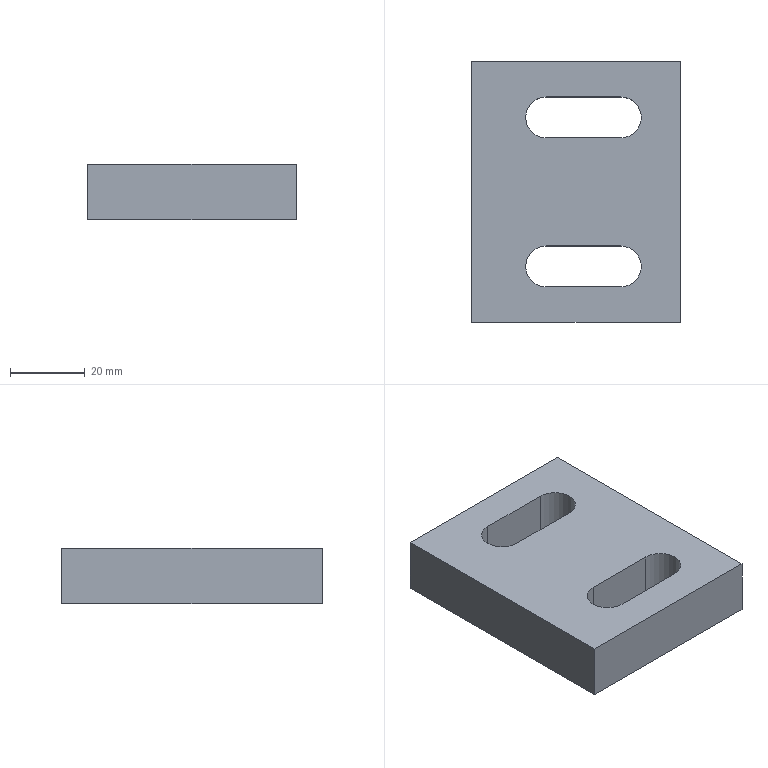Part | 1 solid | 16 faces | box 56 x 70 x 15 mm | volume 49349 mm3 | plane 10 | cylinder 6 | commonest cylinder face diameters 11 x6
STEP:
#1=CARTESIAN_POINT('',(-13.5,20.,15.));
#2=VERTEX_POINT('',#1);
#3=CARTESIAN_POINT('',(-8.,25.5,15.));
#4=VERTEX_POINT('',#3);
#5=CARTESIAN_POINT('',(-8.,20.,15.));
#6=DIRECTION('',(0.,0.,-1.));
#7=DIRECTION('',(-1.,0.,0.));
#8=AXIS2_PLACEMENT_3D('',#5,#6,#7);
#9=CIRCLE('',#8,5.5);
#10=EDGE_CURVE('',#2,#4,#9,.T.);
#11=ORIENTED_EDGE('',*,*,#10,.F.);
#12=CARTESIAN_POINT('',(-13.5,20.,0.));
#13=VERTEX_POINT('',#12);
#14=CARTESIAN_POINT('',(-13.5,20.,15.));
#15=DIRECTION('',(0.,0.,-1.));
#16=VECTOR('',#15,1000.);
#17=LINE('',#14,#16);
#18=EDGE_CURVE('',#2,#13,#17,.T.);
#19=ORIENTED_EDGE('',*,*,#18,.T.);
#20=CARTESIAN_POINT('',(-8.,25.5,0.));
#21=VERTEX_POINT('',#20);
#22=CARTESIAN_POINT('',(-8.,20.,0.));
#23=DIRECTION('',(0.,0.,1.));
#24=DIRECTION('',(-1.,0.,0.));
#25=AXIS2_PLACEMENT_3D('',#22,#23,#24);
#26=CIRCLE('',#25,5.5);
#27=EDGE_CURVE('',#21,#13,#26,.T.);
#28=ORIENTED_EDGE('',*,*,#27,.F.);
#29=CARTESIAN_POINT('',(-8.,25.5,15.));
#30=DIRECTION('',(0.,0.,-1.));
#31=VECTOR('',#30,1000.);
#32=LINE('',#29,#31);
#33=EDGE_CURVE('',#4,#21,#32,.T.);
#34=ORIENTED_EDGE('',*,*,#33,.F.);
#35=EDGE_LOOP('',(#11,#19,#28,#34));
#36=FACE_OUTER_BOUND('',#35,.T.);
#37=CARTESIAN_POINT('',(-8.,20.,15.));
#38=DIRECTION('',(0.,0.,-1.));
#39=DIRECTION('',(-1.,0.,0.));
#40=AXIS2_PLACEMENT_3D('',#37,#38,#39);
#41=CYLINDRICAL_SURFACE('',#40,5.5);
#42=ADVANCED_FACE('',(#36),#41,.F.);
#43=CARTESIAN_POINT('',(-13.5,-20.,15.));
#44=VERTEX_POINT('',#43);
#45=CARTESIAN_POINT('',(-8.,-14.5,15.));
#46=VERTEX_POINT('',#45);
#47=CARTESIAN_POINT('',(-8.,-20.,15.));
#48=DIRECTION('',(0.,0.,-1.));
#49=DIRECTION('',(1.,0.,0.));
#50=AXIS2_PLACEMENT_3D('',#47,#48,#49);
#51=CIRCLE('',#50,5.5);
#52=EDGE_CURVE('',#44,#46,#51,.T.);
#53=ORIENTED_EDGE('',*,*,#52,.F.);
#54=CARTESIAN_POINT('',(-13.5,-20.,0.));
#55=VERTEX_POINT('',#54);
#56=CARTESIAN_POINT('',(-13.5,-20.,15.));
#57=DIRECTION('',(0.,0.,-1.));
#58=VECTOR('',#57,1000.);
#59=LINE('',#56,#58);
#60=EDGE_CURVE('',#44,#55,#59,.T.);
#61=ORIENTED_EDGE('',*,*,#60,.T.);
#62=CARTESIAN_POINT('',(-8.,-14.5,0.));
#63=VERTEX_POINT('',#62);
#64=CARTESIAN_POINT('',(-8.,-20.,0.));
#65=DIRECTION('',(0.,0.,1.));
#66=DIRECTION('',(-1.,0.,0.));
#67=AXIS2_PLACEMENT_3D('',#64,#65,#66);
#68=CIRCLE('',#67,5.5);
#69=EDGE_CURVE('',#63,#55,#68,.T.);
#70=ORIENTED_EDGE('',*,*,#69,.F.);
#71=CARTESIAN_POINT('',(-8.,-14.5,15.));
#72=DIRECTION('',(0.,0.,-1.));
#73=VECTOR('',#72,1000.);
#74=LINE('',#71,#73);
#75=EDGE_CURVE('',#46,#63,#74,.T.);
#76=ORIENTED_EDGE('',*,*,#75,.F.);
#77=EDGE_LOOP('',(#53,#61,#70,#76));
#78=FACE_OUTER_BOUND('',#77,.T.);
#79=CARTESIAN_POINT('',(-8.,-20.,15.));
#80=DIRECTION('',(0.,0.,-1.));
#81=DIRECTION('',(-1.,0.,0.));
#82=AXIS2_PLACEMENT_3D('',#79,#80,#81);
#83=CYLINDRICAL_SURFACE('',#82,5.5);
#84=ADVANCED_FACE('',(#78),#83,.F.);
#85=CARTESIAN_POINT('',(28.,-35.,0.));
#86=VERTEX_POINT('',#85);
#87=CARTESIAN_POINT('',(28.,35.,0.));
#88=VERTEX_POINT('',#87);
#89=CARTESIAN_POINT('',(28.,35.,0.));
#90=DIRECTION('',(0.,1.,0.));
#91=VECTOR('',#90,1000.);
#92=LINE('',#89,#91);
#93=EDGE_CURVE('',#86,#88,#92,.T.);
#94=ORIENTED_EDGE('',*,*,#93,.T.);
#95=CARTESIAN_POINT('',(28.,35.,15.));
#96=VERTEX_POINT('',#95);
#97=CARTESIAN_POINT('',(28.,35.,15.));
#98=DIRECTION('',(0.,0.,-1.));
#99=VECTOR('',#98,1000.);
#100=LINE('',#97,#99);
#101=EDGE_CURVE('',#96,#88,#100,.T.);
#102=ORIENTED_EDGE('',*,*,#101,.F.);
#103=CARTESIAN_POINT('',(28.,-35.,15.));
#104=VERTEX_POINT('',#103);
#105=CARTESIAN_POINT('',(28.,35.,15.));
#106=DIRECTION('',(0.,1.,0.));
#107=VECTOR('',#106,1000.);
#108=LINE('',#105,#107);
#109=EDGE_CURVE('',#104,#96,#108,.T.);
#110=ORIENTED_EDGE('',*,*,#109,.F.);
#111=CARTESIAN_POINT('',(28.,-35.,15.));
#112=DIRECTION('',(0.,0.,-1.));
#113=VECTOR('',#112,1000.);
#114=LINE('',#111,#113);
#115=EDGE_CURVE('',#104,#86,#114,.T.);
#116=ORIENTED_EDGE('',*,*,#115,.T.);
#117=EDGE_LOOP('',(#94,#102,#110,#116));
#118=FACE_OUTER_BOUND('',#117,.T.);
#119=CARTESIAN_POINT('',(28.,35.,15.));
#120=DIRECTION('',(-1.,0.,0.));
#121=DIRECTION('',(0.,-1.,0.));
#122=AXIS2_PLACEMENT_3D('',#119,#120,#121);
#123=PLANE('',#122);
#124=ADVANCED_FACE('',(#118),#123,.F.);
#125=CARTESIAN_POINT('',(-28.,35.,0.));
#126=VERTEX_POINT('',#125);
#127=CARTESIAN_POINT('',(-28.,35.,0.));
#128=DIRECTION('',(-1.,0.,0.));
#129=VECTOR('',#128,1000.);
#130=LINE('',#127,#129);
#131=EDGE_CURVE('',#88,#126,#130,.T.);
#132=ORIENTED_EDGE('',*,*,#131,.T.);
#133=CARTESIAN_POINT('',(-28.,35.,15.));
#134=VERTEX_POINT('',#133);
#135=CARTESIAN_POINT('',(-28.,35.,15.));
#136=DIRECTION('',(0.,0.,-1.));
#137=VECTOR('',#136,1000.);
#138=LINE('',#135,#137);
#139=EDGE_CURVE('',#134,#126,#138,.T.);
#140=ORIENTED_EDGE('',*,*,#139,.F.);
#141=CARTESIAN_POINT('',(-28.,35.,15.));
#142=DIRECTION('',(-1.,0.,0.));
#143=VECTOR('',#142,1000.);
#144=LINE('',#141,#143);
#145=EDGE_CURVE('',#96,#134,#144,.T.);
#146=ORIENTED_EDGE('',*,*,#145,.F.);
#147=ORIENTED_EDGE('',*,*,#101,.T.);
#148=EDGE_LOOP('',(#132,#140,#146,#147));
#149=FACE_OUTER_BOUND('',#148,.T.);
#150=CARTESIAN_POINT('',(-28.,35.,15.));
#151=DIRECTION('',(0.,-1.,0.));
#152=DIRECTION('',(0.,0.,-1.));
#153=AXIS2_PLACEMENT_3D('',#150,#151,#152);
#154=PLANE('',#153);
#155=ADVANCED_FACE('',(#149),#154,.F.);
#156=CARTESIAN_POINT('',(-28.,-35.,0.));
#157=VERTEX_POINT('',#156);
#158=CARTESIAN_POINT('',(-28.,35.,0.));
#159=DIRECTION('',(0.,-1.,0.));
#160=VECTOR('',#159,1000.);
#161=LINE('',#158,#160);
#162=EDGE_CURVE('',#126,#157,#161,.T.);
#163=ORIENTED_EDGE('',*,*,#162,.T.);
#164=CARTESIAN_POINT('',(-28.,-35.,15.));
#165=VERTEX_POINT('',#164);
#166=CARTESIAN_POINT('',(-28.,-35.,15.));
#167=DIRECTION('',(0.,0.,-1.));
#168=VECTOR('',#167,1000.);
#169=LINE('',#166,#168);
#170=EDGE_CURVE('',#165,#157,#169,.T.);
#171=ORIENTED_EDGE('',*,*,#170,.F.);
#172=CARTESIAN_POINT('',(-28.,35.,15.));
#173=DIRECTION('',(0.,-1.,0.));
#174=VECTOR('',#173,1000.);
#175=LINE('',#172,#174);
#176=EDGE_CURVE('',#134,#165,#175,.T.);
#177=ORIENTED_EDGE('',*,*,#176,.F.);
#178=ORIENTED_EDGE('',*,*,#139,.T.);
#179=EDGE_LOOP('',(#163,#171,#177,#178));
#180=FACE_OUTER_BOUND('',#179,.T.);
#181=CARTESIAN_POINT('',(-28.,35.,15.));
#182=DIRECTION('',(1.,0.,0.));
#183=DIRECTION('',(0.,1.,0.));
#184=AXIS2_PLACEMENT_3D('',#181,#182,#183);
#185=PLANE('',#184);
#186=ADVANCED_FACE('',(#180),#185,.F.);
#187=CARTESIAN_POINT('',(-28.,-35.,0.));
#188=DIRECTION('',(1.,0.,0.));
#189=VECTOR('',#188,1000.);
#190=LINE('',#187,#189);
#191=EDGE_CURVE('',#157,#86,#190,.T.);
#192=ORIENTED_EDGE('',*,*,#191,.T.);
#193=ORIENTED_EDGE('',*,*,#115,.F.);
#194=CARTESIAN_POINT('',(-28.,-35.,15.));
#195=DIRECTION('',(1.,0.,0.));
#196=VECTOR('',#195,1000.);
#197=LINE('',#194,#196);
#198=EDGE_CURVE('',#165,#104,#197,.T.);
#199=ORIENTED_EDGE('',*,*,#198,.F.);
#200=ORIENTED_EDGE('',*,*,#170,.T.);
#201=EDGE_LOOP('',(#192,#193,#199,#200));
#202=FACE_OUTER_BOUND('',#201,.T.);
#203=CARTESIAN_POINT('',(-28.,-35.,15.));
#204=DIRECTION('',(0.,1.,0.));
#205=DIRECTION('',(0.,0.,1.));
#206=AXIS2_PLACEMENT_3D('',#203,#204,#205);
#207=PLANE('',#206);
#208=ADVANCED_FACE('',(#202),#207,.F.);
#209=CARTESIAN_POINT('',(12.,25.5,15.));
#210=VERTEX_POINT('',#209);
#211=CARTESIAN_POINT('',(12.,14.5,15.));
#212=VERTEX_POINT('',#211);
#213=CARTESIAN_POINT('',(12.,20.,15.));
#214=DIRECTION('',(0.,0.,-1.));
#215=DIRECTION('',(-1.,0.,0.));
#216=AXIS2_PLACEMENT_3D('',#213,#214,#215);
#217=CIRCLE('',#216,5.5);
#218=EDGE_CURVE('',#210,#212,#217,.T.);
#219=ORIENTED_EDGE('',*,*,#218,.T.);
#220=CARTESIAN_POINT('',(-8.,14.5,15.));
#221=VERTEX_POINT('',#220);
#222=CARTESIAN_POINT('',(12.,14.5,15.));
#223=DIRECTION('',(-1.,0.,0.));
#224=VECTOR('',#223,1000.);
#225=LINE('',#222,#224);
#226=EDGE_CURVE('',#212,#221,#225,.T.);
#227=ORIENTED_EDGE('',*,*,#226,.T.);
#228=CARTESIAN_POINT('',(-8.,20.,15.));
#229=DIRECTION('',(0.,0.,-1.));
#230=DIRECTION('',(-1.,0.,0.));
#231=AXIS2_PLACEMENT_3D('',#228,#229,#230);
#232=CIRCLE('',#231,5.5);
#233=EDGE_CURVE('',#221,#2,#232,.T.);
#234=ORIENTED_EDGE('',*,*,#233,.T.);
#235=ORIENTED_EDGE('',*,*,#10,.T.);
#236=CARTESIAN_POINT('',(12.,25.5,15.));
#237=DIRECTION('',(1.,0.,0.));
#238=VECTOR('',#237,1000.);
#239=LINE('',#236,#238);
#240=EDGE_CURVE('',#4,#210,#239,.T.);
#241=ORIENTED_EDGE('',*,*,#240,.T.);
#242=EDGE_LOOP('',(#219,#227,#234,#235,#241));
#243=FACE_BOUND('',#242,.T.);
#244=CARTESIAN_POINT('',(12.,-14.5,15.));
#245=VERTEX_POINT('',#244);
#246=CARTESIAN_POINT('',(12.,-25.5,15.));
#247=VERTEX_POINT('',#246);
#248=CARTESIAN_POINT('',(12.,-20.,15.));
#249=DIRECTION('',(0.,0.,-1.));
#250=DIRECTION('',(1.,0.,0.));
#251=AXIS2_PLACEMENT_3D('',#248,#249,#250);
#252=CIRCLE('',#251,5.5);
#253=EDGE_CURVE('',#245,#247,#252,.T.);
#254=ORIENTED_EDGE('',*,*,#253,.T.);
#255=CARTESIAN_POINT('',(-8.,-25.5,15.));
#256=VERTEX_POINT('',#255);
#257=CARTESIAN_POINT('',(12.,-25.5,15.));
#258=DIRECTION('',(-1.,0.,0.));
#259=VECTOR('',#258,1000.);
#260=LINE('',#257,#259);
#261=EDGE_CURVE('',#247,#256,#260,.T.);
#262=ORIENTED_EDGE('',*,*,#261,.T.);
#263=CARTESIAN_POINT('',(-8.,-20.,15.));
#264=DIRECTION('',(0.,0.,-1.));
#265=DIRECTION('',(1.,0.,0.));
#266=AXIS2_PLACEMENT_3D('',#263,#264,#265);
#267=CIRCLE('',#266,5.5);
#268=EDGE_CURVE('',#256,#44,#267,.T.);
#269=ORIENTED_EDGE('',*,*,#268,.T.);
#270=ORIENTED_EDGE('',*,*,#52,.T.);
#271=CARTESIAN_POINT('',(12.,-14.5,15.));
#272=DIRECTION('',(1.,0.,0.));
#273=VECTOR('',#272,1000.);
#274=LINE('',#271,#273);
#275=EDGE_CURVE('',#46,#245,#274,.T.);
#276=ORIENTED_EDGE('',*,*,#275,.T.);
#277=EDGE_LOOP('',(#254,#262,#269,#270,#276));
#278=FACE_BOUND('',#277,.T.);
#279=ORIENTED_EDGE('',*,*,#109,.T.);
#280=ORIENTED_EDGE('',*,*,#145,.T.);
#281=ORIENTED_EDGE('',*,*,#176,.T.);
#282=ORIENTED_EDGE('',*,*,#198,.T.);
#283=EDGE_LOOP('',(#279,#280,#281,#282));
#284=FACE_OUTER_BOUND('',#283,.T.);
#285=CARTESIAN_POINT('',(0.,0.,15.));
#286=DIRECTION('',(0.,0.,1.));
#287=DIRECTION('',(1.,0.,0.));
#288=AXIS2_PLACEMENT_3D('',#285,#286,#287);
#289=PLANE('',#288);
#290=ADVANCED_FACE('',(#243,#278,#284),#289,.T.);
#291=CARTESIAN_POINT('',(-8.,14.5,0.));
#292=VERTEX_POINT('',#291);
#293=CARTESIAN_POINT('',(12.,14.5,0.));
#294=VERTEX_POINT('',#293);
#295=CARTESIAN_POINT('',(0.,14.5,0.));
#296=DIRECTION('',(1.,0.,0.));
#297=VECTOR('',#296,1000.);
#298=LINE('',#295,#297);
#299=EDGE_CURVE('',#292,#294,#298,.T.);
#300=ORIENTED_EDGE('',*,*,#299,.T.);
#301=CARTESIAN_POINT('',(12.,25.5,0.));
#302=VERTEX_POINT('',#301);
#303=CARTESIAN_POINT('',(12.,20.,0.));
#304=DIRECTION('',(0.,0.,1.));
#305=DIRECTION('',(-1.,0.,0.));
#306=AXIS2_PLACEMENT_3D('',#303,#304,#305);
#307=CIRCLE('',#306,5.5);
#308=EDGE_CURVE('',#294,#302,#307,.T.);
#309=ORIENTED_EDGE('',*,*,#308,.T.);
#310=CARTESIAN_POINT('',(0.,25.5,0.));
#311=DIRECTION('',(-1.,0.,0.));
#312=VECTOR('',#311,1000.);
#313=LINE('',#310,#312);
#314=EDGE_CURVE('',#302,#21,#313,.T.);
#315=ORIENTED_EDGE('',*,*,#314,.T.);
#316=ORIENTED_EDGE('',*,*,#27,.T.);
#317=CARTESIAN_POINT('',(-8.,20.,0.));
#318=DIRECTION('',(0.,0.,1.));
#319=DIRECTION('',(-1.,0.,0.));
#320=AXIS2_PLACEMENT_3D('',#317,#318,#319);
#321=CIRCLE('',#320,5.5);
#322=EDGE_CURVE('',#13,#292,#321,.T.);
#323=ORIENTED_EDGE('',*,*,#322,.T.);
#324=EDGE_LOOP('',(#300,#309,#315,#316,#323));
#325=FACE_BOUND('',#324,.T.);
#326=CARTESIAN_POINT('',(-8.,-25.5,0.));
#327=VERTEX_POINT('',#326);
#328=CARTESIAN_POINT('',(12.,-25.5,0.));
#329=VERTEX_POINT('',#328);
#330=CARTESIAN_POINT('',(0.,-25.5,0.));
#331=DIRECTION('',(1.,0.,0.));
#332=VECTOR('',#331,1000.);
#333=LINE('',#330,#332);
#334=EDGE_CURVE('',#327,#329,#333,.T.);
#335=ORIENTED_EDGE('',*,*,#334,.T.);
#336=CARTESIAN_POINT('',(12.,-14.5,0.));
#337=VERTEX_POINT('',#336);
#338=CARTESIAN_POINT('',(12.,-20.,0.));
#339=DIRECTION('',(0.,0.,1.));
#340=DIRECTION('',(-1.,0.,0.));
#341=AXIS2_PLACEMENT_3D('',#338,#339,#340);
#342=CIRCLE('',#341,5.5);
#343=EDGE_CURVE('',#329,#337,#342,.T.);
#344=ORIENTED_EDGE('',*,*,#343,.T.);
#345=CARTESIAN_POINT('',(0.,-14.5,0.));
#346=DIRECTION('',(-1.,0.,0.));
#347=VECTOR('',#346,1000.);
#348=LINE('',#345,#347);
#349=EDGE_CURVE('',#337,#63,#348,.T.);
#350=ORIENTED_EDGE('',*,*,#349,.T.);
#351=ORIENTED_EDGE('',*,*,#69,.T.);
#352=CARTESIAN_POINT('',(-8.,-20.,0.));
#353=DIRECTION('',(0.,0.,1.));
#354=DIRECTION('',(-1.,0.,0.));
#355=AXIS2_PLACEMENT_3D('',#352,#353,#354);
#356=CIRCLE('',#355,5.5);
#357=EDGE_CURVE('',#55,#327,#356,.T.);
#358=ORIENTED_EDGE('',*,*,#357,.T.);
#359=EDGE_LOOP('',(#335,#344,#350,#351,#358));
#360=FACE_BOUND('',#359,.T.);
#361=ORIENTED_EDGE('',*,*,#93,.F.);
#362=ORIENTED_EDGE('',*,*,#191,.F.);
#363=ORIENTED_EDGE('',*,*,#162,.F.);
#364=ORIENTED_EDGE('',*,*,#131,.F.);
#365=EDGE_LOOP('',(#361,#362,#363,#364));
#366=FACE_OUTER_BOUND('',#365,.T.);
#367=CARTESIAN_POINT('',(0.,0.,0.));
#368=DIRECTION('',(0.,0.,1.));
#369=DIRECTION('',(1.,0.,0.));
#370=AXIS2_PLACEMENT_3D('',#367,#368,#369);
#371=PLANE('',#370);
#372=ADVANCED_FACE('',(#325,#360,#366),#371,.F.);
#373=CARTESIAN_POINT('',(12.,-25.5,15.));
#374=DIRECTION('',(0.,0.,-1.));
#375=VECTOR('',#374,1000.);
#376=LINE('',#373,#375);
#377=EDGE_CURVE('',#247,#329,#376,.T.);
#378=ORIENTED_EDGE('',*,*,#377,.F.);
#379=ORIENTED_EDGE('',*,*,#253,.F.);
#380=CARTESIAN_POINT('',(12.,-14.5,15.));
#381=DIRECTION('',(0.,0.,-1.));
#382=VECTOR('',#381,1000.);
#383=LINE('',#380,#382);
#384=EDGE_CURVE('',#245,#337,#383,.T.);
#385=ORIENTED_EDGE('',*,*,#384,.T.);
#386=ORIENTED_EDGE('',*,*,#343,.F.);
#387=EDGE_LOOP('',(#378,#379,#385,#386));
#388=FACE_OUTER_BOUND('',#387,.T.);
#389=CARTESIAN_POINT('',(12.,-20.,15.));
#390=DIRECTION('',(0.,0.,-1.));
#391=DIRECTION('',(-1.,0.,0.));
#392=AXIS2_PLACEMENT_3D('',#389,#390,#391);
#393=CYLINDRICAL_SURFACE('',#392,5.5);
#394=ADVANCED_FACE('',(#388),#393,.F.);
#395=ORIENTED_EDGE('',*,*,#384,.F.);
#396=ORIENTED_EDGE('',*,*,#275,.F.);
#397=ORIENTED_EDGE('',*,*,#75,.T.);
#398=ORIENTED_EDGE('',*,*,#349,.F.);
#399=EDGE_LOOP('',(#395,#396,#397,#398));
#400=FACE_OUTER_BOUND('',#399,.T.);
#401=CARTESIAN_POINT('',(12.,-14.5,15.));
#402=DIRECTION('',(0.,1.,0.));
#403=DIRECTION('',(-1.,0.,0.));
#404=AXIS2_PLACEMENT_3D('',#401,#402,#403);
#405=PLANE('',#404);
#406=ADVANCED_FACE('',(#400),#405,.F.);
#407=ORIENTED_EDGE('',*,*,#60,.F.);
#408=ORIENTED_EDGE('',*,*,#268,.F.);
#409=CARTESIAN_POINT('',(-8.,-25.5,15.));
#410=DIRECTION('',(0.,0.,-1.));
#411=VECTOR('',#410,1000.);
#412=LINE('',#409,#411);
#413=EDGE_CURVE('',#256,#327,#412,.T.);
#414=ORIENTED_EDGE('',*,*,#413,.T.);
#415=ORIENTED_EDGE('',*,*,#357,.F.);
#416=EDGE_LOOP('',(#407,#408,#414,#415));
#417=FACE_OUTER_BOUND('',#416,.T.);
#418=CARTESIAN_POINT('',(-8.,-20.,15.));
#419=DIRECTION('',(0.,0.,-1.));
#420=DIRECTION('',(-1.,0.,0.));
#421=AXIS2_PLACEMENT_3D('',#418,#419,#420);
#422=CYLINDRICAL_SURFACE('',#421,5.5);
#423=ADVANCED_FACE('',(#417),#422,.F.);
#424=ORIENTED_EDGE('',*,*,#413,.F.);
#425=ORIENTED_EDGE('',*,*,#261,.F.);
#426=ORIENTED_EDGE('',*,*,#377,.T.);
#427=ORIENTED_EDGE('',*,*,#334,.F.);
#428=EDGE_LOOP('',(#424,#425,#426,#427));
#429=FACE_OUTER_BOUND('',#428,.T.);
#430=CARTESIAN_POINT('',(12.,-25.5,15.));
#431=DIRECTION('',(0.,-1.,0.));
#432=DIRECTION('',(1.,0.,0.));
#433=AXIS2_PLACEMENT_3D('',#430,#431,#432);
#434=PLANE('',#433);
#435=ADVANCED_FACE('',(#429),#434,.F.);
#436=CARTESIAN_POINT('',(12.,14.5,15.));
#437=DIRECTION('',(0.,0.,-1.));
#438=VECTOR('',#437,1000.);
#439=LINE('',#436,#438);
#440=EDGE_CURVE('',#212,#294,#439,.T.);
#441=ORIENTED_EDGE('',*,*,#440,.F.);
#442=ORIENTED_EDGE('',*,*,#218,.F.);
#443=CARTESIAN_POINT('',(12.,25.5,15.));
#444=DIRECTION('',(0.,0.,-1.));
#445=VECTOR('',#444,1000.);
#446=LINE('',#443,#445);
#447=EDGE_CURVE('',#210,#302,#446,.T.);
#448=ORIENTED_EDGE('',*,*,#447,.T.);
#449=ORIENTED_EDGE('',*,*,#308,.F.);
#450=EDGE_LOOP('',(#441,#442,#448,#449));
#451=FACE_OUTER_BOUND('',#450,.T.);
#452=CARTESIAN_POINT('',(12.,20.,15.));
#453=DIRECTION('',(0.,0.,-1.));
#454=DIRECTION('',(-1.,0.,0.));
#455=AXIS2_PLACEMENT_3D('',#452,#453,#454);
#456=CYLINDRICAL_SURFACE('',#455,5.5);
#457=ADVANCED_FACE('',(#451),#456,.F.);
#458=ORIENTED_EDGE('',*,*,#447,.F.);
#459=ORIENTED_EDGE('',*,*,#240,.F.);
#460=ORIENTED_EDGE('',*,*,#33,.T.);
#461=ORIENTED_EDGE('',*,*,#314,.F.);
#462=EDGE_LOOP('',(#458,#459,#460,#461));
#463=FACE_OUTER_BOUND('',#462,.T.);
#464=CARTESIAN_POINT('',(12.,25.5,15.));
#465=DIRECTION('',(0.,1.,0.));
#466=DIRECTION('',(-1.,0.,0.));
#467=AXIS2_PLACEMENT_3D('',#464,#465,#466);
#468=PLANE('',#467);
#469=ADVANCED_FACE('',(#463),#468,.F.);
#470=ORIENTED_EDGE('',*,*,#18,.F.);
#471=ORIENTED_EDGE('',*,*,#233,.F.);
#472=CARTESIAN_POINT('',(-8.,14.5,15.));
#473=DIRECTION('',(0.,0.,-1.));
#474=VECTOR('',#473,1000.);
#475=LINE('',#472,#474);
#476=EDGE_CURVE('',#221,#292,#475,.T.);
#477=ORIENTED_EDGE('',*,*,#476,.T.);
#478=ORIENTED_EDGE('',*,*,#322,.F.);
#479=EDGE_LOOP('',(#470,#471,#477,#478));
#480=FACE_OUTER_BOUND('',#479,.T.);
#481=CARTESIAN_POINT('',(-8.,20.,15.));
#482=DIRECTION('',(0.,0.,-1.));
#483=DIRECTION('',(-1.,0.,0.));
#484=AXIS2_PLACEMENT_3D('',#481,#482,#483);
#485=CYLINDRICAL_SURFACE('',#484,5.5);
#486=ADVANCED_FACE('',(#480),#485,.F.);
#487=ORIENTED_EDGE('',*,*,#476,.F.);
#488=ORIENTED_EDGE('',*,*,#226,.F.);
#489=ORIENTED_EDGE('',*,*,#440,.T.);
#490=ORIENTED_EDGE('',*,*,#299,.F.);
#491=EDGE_LOOP('',(#487,#488,#489,#490));
#492=FACE_OUTER_BOUND('',#491,.T.);
#493=CARTESIAN_POINT('',(12.,14.5,15.));
#494=DIRECTION('',(0.,-1.,0.));
#495=DIRECTION('',(1.,0.,0.));
#496=AXIS2_PLACEMENT_3D('',#493,#494,#495);
#497=PLANE('',#496);
#498=ADVANCED_FACE('',(#492),#497,.F.);
#499=CLOSED_SHELL('',(#42,#84,#124,#155,#186,#208,#290,#372,#394,#406,#423,#435,#457,#469,#486,#498));
#500=MANIFOLD_SOLID_BREP('',#499);
#501=CARTESIAN_POINT('',(0.,0.,0.));
#502=DIRECTION('',(0.,0.,1.));
#503=DIRECTION('',(1.,0.,0.));
#504=AXIS2_PLACEMENT_3D('',#501,#502,#503);
#505=(LENGTH_UNIT()NAMED_UNIT(*)SI_UNIT(.MILLI.,.METRE.));
#506=UNCERTAINTY_MEASURE_WITH_UNIT(LENGTH_MEASURE(0.00001),#505,'','');
#507=(NAMED_UNIT(*)PLANE_ANGLE_UNIT()SI_UNIT($,.RADIAN.));
#508=(NAMED_UNIT(*)SI_UNIT($,.STERADIAN.)SOLID_ANGLE_UNIT());
#509=(GEOMETRIC_REPRESENTATION_CONTEXT(3)GLOBAL_UNCERTAINTY_ASSIGNED_CONTEXT((#506))GLOBAL_UNIT_ASSIGNED_CONTEXT((#505,#507,#508))REPRESENTATION_CONTEXT('',''));
#510=ADVANCED_BREP_SHAPE_REPRESENTATION('',(#500,#504),#509);